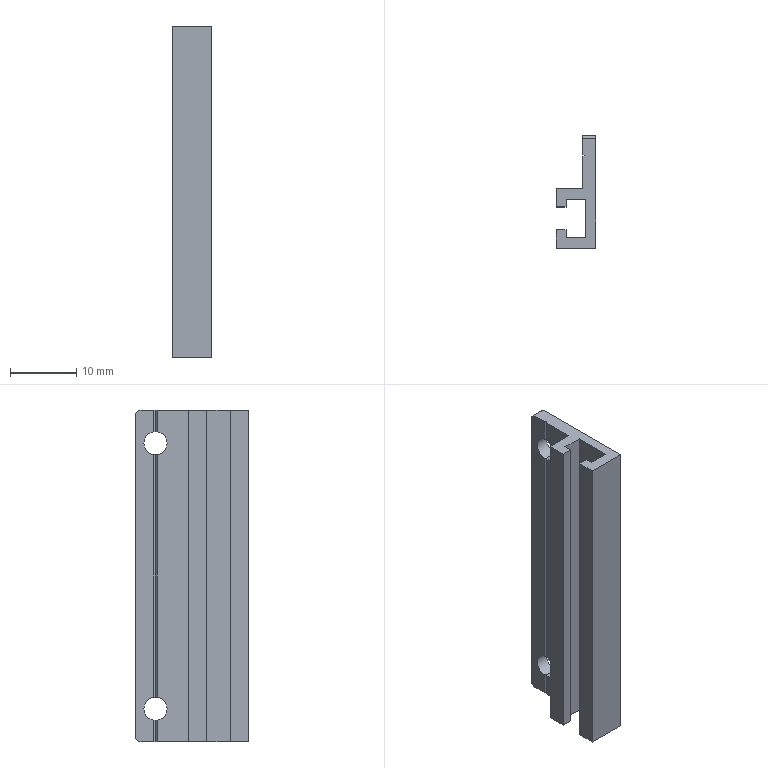Part | STEP file | PN_0026 Sensor BKT | 1 solid | 29 faces | box 6 x 17 x 50 mm | volume 2341 mm3 | plane 25 | cylinder 4 | commonest cylinder face diameters 3.5 x4